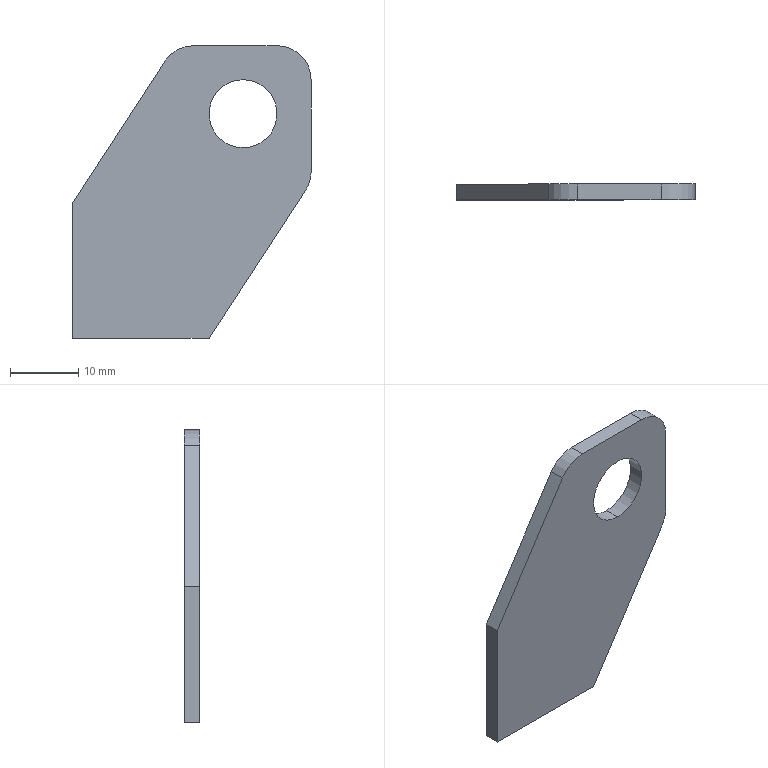Part | SolidWorks | features FlatPattern 1, SMBaseFlange 1, SheetMetal 1 | 1 solid | 13 faces | box 35 x 2.3 x 43 mm | volume 2472 mm3 | plane 8 | cylinder 5 | commonest cylinder face diameters 10 x5
STEP:
#1=CARTESIAN_POINT('',(25.,-2.3,28.));
#2=VERTEX_POINT('',#1);
#3=CARTESIAN_POINT('',(25.,-2.3,38.));
#4=VERTEX_POINT('',#3);
#5=CARTESIAN_POINT('',(25.,-2.3,33.));
#6=DIRECTION('',(0.,1.,0.));
#7=DIRECTION('',(0.,0.,1.));
#8=AXIS2_PLACEMENT_3D('',#5,#6,#7);
#9=CIRCLE('',#8,5.);
#10=EDGE_CURVE('',#2,#4,#9,.T.);
#11=ORIENTED_EDGE('',*,*,#10,.F.);
#12=CARTESIAN_POINT('',(25.,0.,28.));
#13=VERTEX_POINT('',#12);
#14=CARTESIAN_POINT('',(25.,-2.3,28.));
#15=DIRECTION('',(0.,1.,0.));
#16=VECTOR('',#15,1000.);
#17=LINE('',#14,#16);
#18=EDGE_CURVE('',#2,#13,#17,.T.);
#19=ORIENTED_EDGE('',*,*,#18,.T.);
#20=CARTESIAN_POINT('',(25.,0.,38.));
#21=VERTEX_POINT('',#20);
#22=CARTESIAN_POINT('',(25.,0.,33.));
#23=DIRECTION('',(0.,1.,0.));
#24=DIRECTION('',(0.,0.,1.));
#25=AXIS2_PLACEMENT_3D('',#22,#23,#24);
#26=CIRCLE('',#25,5.);
#27=EDGE_CURVE('',#13,#21,#26,.T.);
#28=ORIENTED_EDGE('',*,*,#27,.T.);
#29=CARTESIAN_POINT('',(25.,-2.3,38.));
#30=DIRECTION('',(0.,1.,0.));
#31=VECTOR('',#30,1000.);
#32=LINE('',#29,#31);
#33=EDGE_CURVE('',#4,#21,#32,.T.);
#34=ORIENTED_EDGE('',*,*,#33,.F.);
#35=EDGE_LOOP('',(#11,#19,#28,#34));
#36=FACE_OUTER_BOUND('',#35,.T.);
#37=CARTESIAN_POINT('',(25.,-2.3,33.));
#38=DIRECTION('',(0.,1.,0.));
#39=DIRECTION('',(0.,0.,1.));
#40=AXIS2_PLACEMENT_3D('',#37,#38,#39);
#41=CYLINDRICAL_SURFACE('',#40,5.);
#42=ADVANCED_FACE('',(#36),#41,.F.);
#43=CARTESIAN_POINT('',(0.,0.,0.));
#44=VERTEX_POINT('',#43);
#45=CARTESIAN_POINT('',(0.,0.,20.));
#46=VERTEX_POINT('',#45);
#47=CARTESIAN_POINT('',(0.,0.,0.));
#48=DIRECTION('',(0.,0.,1.));
#49=VECTOR('',#48,1000.);
#50=LINE('',#47,#49);
#51=EDGE_CURVE('',#44,#46,#50,.T.);
#52=ORIENTED_EDGE('',*,*,#51,.F.);
#53=CARTESIAN_POINT('',(0.,-2.3,0.));
#54=VERTEX_POINT('',#53);
#55=CARTESIAN_POINT('',(0.,-2.3,0.));
#56=DIRECTION('',(0.,1.,0.));
#57=VECTOR('',#56,1000.);
#58=LINE('',#55,#57);
#59=EDGE_CURVE('',#54,#44,#58,.T.);
#60=ORIENTED_EDGE('',*,*,#59,.F.);
#61=CARTESIAN_POINT('',(0.,-2.3,20.));
#62=VERTEX_POINT('',#61);
#63=CARTESIAN_POINT('',(0.,-2.3,0.));
#64=DIRECTION('',(0.,0.,1.));
#65=VECTOR('',#64,1000.);
#66=LINE('',#63,#65);
#67=EDGE_CURVE('',#54,#62,#66,.T.);
#68=ORIENTED_EDGE('',*,*,#67,.T.);
#69=CARTESIAN_POINT('',(0.,-2.3,20.));
#70=DIRECTION('',(0.,1.,0.));
#71=VECTOR('',#70,1000.);
#72=LINE('',#69,#71);
#73=EDGE_CURVE('',#62,#46,#72,.T.);
#74=ORIENTED_EDGE('',*,*,#73,.T.);
#75=EDGE_LOOP('',(#52,#60,#68,#74));
#76=FACE_OUTER_BOUND('',#75,.T.);
#77=CARTESIAN_POINT('',(0.,-2.3,0.));
#78=DIRECTION('',(-1.,0.,0.));
#79=DIRECTION('',(0.,0.,1.));
#80=AXIS2_PLACEMENT_3D('',#77,#78,#79);
#81=PLANE('',#80);
#82=ADVANCED_FACE('',(#76),#81,.T.);
#83=CARTESIAN_POINT('',(20.,0.,0.));
#84=VERTEX_POINT('',#83);
#85=CARTESIAN_POINT('',(0.,0.,0.));
#86=DIRECTION('',(-1.,0.,0.));
#87=VECTOR('',#86,1000.);
#88=LINE('',#85,#87);
#89=EDGE_CURVE('',#84,#44,#88,.T.);
#90=ORIENTED_EDGE('',*,*,#89,.F.);
#91=CARTESIAN_POINT('',(20.,-2.3,0.));
#92=VERTEX_POINT('',#91);
#93=CARTESIAN_POINT('',(20.,-2.3,0.));
#94=DIRECTION('',(0.,1.,0.));
#95=VECTOR('',#94,1000.);
#96=LINE('',#93,#95);
#97=EDGE_CURVE('',#92,#84,#96,.T.);
#98=ORIENTED_EDGE('',*,*,#97,.F.);
#99=CARTESIAN_POINT('',(0.,-2.3,0.));
#100=DIRECTION('',(-1.,0.,0.));
#101=VECTOR('',#100,1000.);
#102=LINE('',#99,#101);
#103=EDGE_CURVE('',#92,#54,#102,.T.);
#104=ORIENTED_EDGE('',*,*,#103,.T.);
#105=ORIENTED_EDGE('',*,*,#59,.T.);
#106=EDGE_LOOP('',(#90,#98,#104,#105));
#107=FACE_OUTER_BOUND('',#106,.T.);
#108=CARTESIAN_POINT('',(0.,-2.3,0.));
#109=DIRECTION('',(0.,0.,-1.));
#110=DIRECTION('',(-1.,0.,0.));
#111=AXIS2_PLACEMENT_3D('',#108,#109,#110);
#112=PLANE('',#111);
#113=ADVANCED_FACE('',(#107),#112,.T.);
#114=CARTESIAN_POINT('',(34.188,0.,21.755));
#115=VERTEX_POINT('',#114);
#116=CARTESIAN_POINT('',(20.,0.,0.));
#117=DIRECTION('',(-0.5463,0.,-0.8376));
#118=VECTOR('',#117,1000.);
#119=LINE('',#116,#118);
#120=EDGE_CURVE('',#115,#84,#119,.T.);
#121=ORIENTED_EDGE('',*,*,#120,.F.);
#122=CARTESIAN_POINT('',(34.188,-2.3,21.755));
#123=VERTEX_POINT('',#122);
#124=CARTESIAN_POINT('',(34.188,-2.3,21.755));
#125=DIRECTION('',(0.,1.,0.));
#126=VECTOR('',#125,1000.);
#127=LINE('',#124,#126);
#128=EDGE_CURVE('',#123,#115,#127,.T.);
#129=ORIENTED_EDGE('',*,*,#128,.F.);
#130=CARTESIAN_POINT('',(20.,-2.3,0.));
#131=DIRECTION('',(-0.5463,0.,-0.8376));
#132=VECTOR('',#131,1000.);
#133=LINE('',#130,#132);
#134=EDGE_CURVE('',#123,#92,#133,.T.);
#135=ORIENTED_EDGE('',*,*,#134,.T.);
#136=ORIENTED_EDGE('',*,*,#97,.T.);
#137=EDGE_LOOP('',(#121,#129,#135,#136));
#138=FACE_OUTER_BOUND('',#137,.T.);
#139=CARTESIAN_POINT('',(20.,-2.3,0.));
#140=DIRECTION('',(0.8376,0.,-0.5463));
#141=DIRECTION('',(-0.5463,0.,-0.8376));
#142=AXIS2_PLACEMENT_3D('',#139,#140,#141);
#143=PLANE('',#142);
#144=ADVANCED_FACE('',(#138),#143,.T.);
#145=CARTESIAN_POINT('',(35.,0.,24.486));
#146=VERTEX_POINT('',#145);
#147=CARTESIAN_POINT('',(30.,0.,24.486));
#148=DIRECTION('',(0.,1.,0.));
#149=DIRECTION('',(0.,0.,-1.));
#150=AXIS2_PLACEMENT_3D('',#147,#148,#149);
#151=CIRCLE('',#150,5.);
#152=EDGE_CURVE('',#146,#115,#151,.T.);
#153=ORIENTED_EDGE('',*,*,#152,.F.);
#154=CARTESIAN_POINT('',(35.,-2.3,24.486));
#155=VERTEX_POINT('',#154);
#156=CARTESIAN_POINT('',(35.,-2.3,24.486));
#157=DIRECTION('',(0.,1.,0.));
#158=VECTOR('',#157,1000.);
#159=LINE('',#156,#158);
#160=EDGE_CURVE('',#155,#146,#159,.T.);
#161=ORIENTED_EDGE('',*,*,#160,.F.);
#162=CARTESIAN_POINT('',(30.,-2.3,24.486));
#163=DIRECTION('',(0.,1.,0.));
#164=DIRECTION('',(0.,0.,-1.));
#165=AXIS2_PLACEMENT_3D('',#162,#163,#164);
#166=CIRCLE('',#165,5.);
#167=EDGE_CURVE('',#155,#123,#166,.T.);
#168=ORIENTED_EDGE('',*,*,#167,.T.);
#169=ORIENTED_EDGE('',*,*,#128,.T.);
#170=EDGE_LOOP('',(#153,#161,#168,#169));
#171=FACE_OUTER_BOUND('',#170,.T.);
#172=CARTESIAN_POINT('',(30.,-2.3,24.486));
#173=DIRECTION('',(0.,1.,0.));
#174=DIRECTION('',(0.,0.,1.));
#175=AXIS2_PLACEMENT_3D('',#172,#173,#174);
#176=CYLINDRICAL_SURFACE('',#175,5.);
#177=ADVANCED_FACE('',(#171),#176,.T.);
#178=CARTESIAN_POINT('',(35.,0.,38.));
#179=VERTEX_POINT('',#178);
#180=CARTESIAN_POINT('',(35.,0.,24.486));
#181=DIRECTION('',(0.,0.,-1.));
#182=VECTOR('',#181,1000.);
#183=LINE('',#180,#182);
#184=EDGE_CURVE('',#179,#146,#183,.T.);
#185=ORIENTED_EDGE('',*,*,#184,.F.);
#186=CARTESIAN_POINT('',(35.,-2.3,38.));
#187=VERTEX_POINT('',#186);
#188=CARTESIAN_POINT('',(35.,-2.3,38.));
#189=DIRECTION('',(0.,1.,0.));
#190=VECTOR('',#189,1000.);
#191=LINE('',#188,#190);
#192=EDGE_CURVE('',#187,#179,#191,.T.);
#193=ORIENTED_EDGE('',*,*,#192,.F.);
#194=CARTESIAN_POINT('',(35.,-2.3,24.486));
#195=DIRECTION('',(0.,0.,-1.));
#196=VECTOR('',#195,1000.);
#197=LINE('',#194,#196);
#198=EDGE_CURVE('',#187,#155,#197,.T.);
#199=ORIENTED_EDGE('',*,*,#198,.T.);
#200=ORIENTED_EDGE('',*,*,#160,.T.);
#201=EDGE_LOOP('',(#185,#193,#199,#200));
#202=FACE_OUTER_BOUND('',#201,.T.);
#203=CARTESIAN_POINT('',(35.,-2.3,24.486));
#204=DIRECTION('',(1.,0.,0.));
#205=DIRECTION('',(0.,0.,-1.));
#206=AXIS2_PLACEMENT_3D('',#203,#204,#205);
#207=PLANE('',#206);
#208=ADVANCED_FACE('',(#202),#207,.T.);
#209=CARTESIAN_POINT('',(30.,0.,43.));
#210=VERTEX_POINT('',#209);
#211=CARTESIAN_POINT('',(30.,0.,38.));
#212=DIRECTION('',(0.,1.,0.));
#213=DIRECTION('',(0.,0.,1.));
#214=AXIS2_PLACEMENT_3D('',#211,#212,#213);
#215=CIRCLE('',#214,5.);
#216=EDGE_CURVE('',#210,#179,#215,.T.);
#217=ORIENTED_EDGE('',*,*,#216,.F.);
#218=CARTESIAN_POINT('',(30.,-2.3,43.));
#219=VERTEX_POINT('',#218);
#220=CARTESIAN_POINT('',(30.,-2.3,43.));
#221=DIRECTION('',(0.,1.,0.));
#222=VECTOR('',#221,1000.);
#223=LINE('',#220,#222);
#224=EDGE_CURVE('',#219,#210,#223,.T.);
#225=ORIENTED_EDGE('',*,*,#224,.F.);
#226=CARTESIAN_POINT('',(30.,-2.3,38.));
#227=DIRECTION('',(0.,1.,0.));
#228=DIRECTION('',(0.,0.,1.));
#229=AXIS2_PLACEMENT_3D('',#226,#227,#228);
#230=CIRCLE('',#229,5.);
#231=EDGE_CURVE('',#219,#187,#230,.T.);
#232=ORIENTED_EDGE('',*,*,#231,.T.);
#233=ORIENTED_EDGE('',*,*,#192,.T.);
#234=EDGE_LOOP('',(#217,#225,#232,#233));
#235=FACE_OUTER_BOUND('',#234,.T.);
#236=CARTESIAN_POINT('',(30.,-2.3,38.));
#237=DIRECTION('',(0.,1.,0.));
#238=DIRECTION('',(0.,0.,1.));
#239=AXIS2_PLACEMENT_3D('',#236,#237,#238);
#240=CYLINDRICAL_SURFACE('',#239,5.);
#241=ADVANCED_FACE('',(#235),#240,.T.);
#242=CARTESIAN_POINT('',(17.708,0.,43.));
#243=VERTEX_POINT('',#242);
#244=CARTESIAN_POINT('',(17.708,0.,43.));
#245=DIRECTION('',(1.,0.,0.));
#246=VECTOR('',#245,1000.);
#247=LINE('',#244,#246);
#248=EDGE_CURVE('',#243,#210,#247,.T.);
#249=ORIENTED_EDGE('',*,*,#248,.F.);
#250=CARTESIAN_POINT('',(17.708,-2.3,43.));
#251=VERTEX_POINT('',#250);
#252=CARTESIAN_POINT('',(17.708,-2.3,43.));
#253=DIRECTION('',(0.,1.,0.));
#254=VECTOR('',#253,1000.);
#255=LINE('',#252,#254);
#256=EDGE_CURVE('',#251,#243,#255,.T.);
#257=ORIENTED_EDGE('',*,*,#256,.F.);
#258=CARTESIAN_POINT('',(17.708,-2.3,43.));
#259=DIRECTION('',(1.,0.,0.));
#260=VECTOR('',#259,1000.);
#261=LINE('',#258,#260);
#262=EDGE_CURVE('',#251,#219,#261,.T.);
#263=ORIENTED_EDGE('',*,*,#262,.T.);
#264=ORIENTED_EDGE('',*,*,#224,.T.);
#265=EDGE_LOOP('',(#249,#257,#263,#264));
#266=FACE_OUTER_BOUND('',#265,.T.);
#267=CARTESIAN_POINT('',(17.708,-2.3,43.));
#268=DIRECTION('',(0.,0.,1.));
#269=DIRECTION('',(1.,0.,0.));
#270=AXIS2_PLACEMENT_3D('',#267,#268,#269);
#271=PLANE('',#270);
#272=ADVANCED_FACE('',(#266),#271,.T.);
#273=CARTESIAN_POINT('',(13.52,0.,40.731));
#274=VERTEX_POINT('',#273);
#275=CARTESIAN_POINT('',(17.708,0.,38.));
#276=DIRECTION('',(0.,1.,0.));
#277=DIRECTION('',(0.,0.,-1.));
#278=AXIS2_PLACEMENT_3D('',#275,#276,#277);
#279=CIRCLE('',#278,5.);
#280=EDGE_CURVE('',#274,#243,#279,.T.);
#281=ORIENTED_EDGE('',*,*,#280,.F.);
#282=CARTESIAN_POINT('',(13.52,-2.3,40.731));
#283=VERTEX_POINT('',#282);
#284=CARTESIAN_POINT('',(13.52,-2.3,40.731));
#285=DIRECTION('',(0.,1.,0.));
#286=VECTOR('',#285,1000.);
#287=LINE('',#284,#286);
#288=EDGE_CURVE('',#283,#274,#287,.T.);
#289=ORIENTED_EDGE('',*,*,#288,.F.);
#290=CARTESIAN_POINT('',(17.708,-2.3,38.));
#291=DIRECTION('',(0.,1.,0.));
#292=DIRECTION('',(0.,0.,-1.));
#293=AXIS2_PLACEMENT_3D('',#290,#291,#292);
#294=CIRCLE('',#293,5.);
#295=EDGE_CURVE('',#283,#251,#294,.T.);
#296=ORIENTED_EDGE('',*,*,#295,.T.);
#297=ORIENTED_EDGE('',*,*,#256,.T.);
#298=EDGE_LOOP('',(#281,#289,#296,#297));
#299=FACE_OUTER_BOUND('',#298,.T.);
#300=CARTESIAN_POINT('',(17.708,-2.3,38.));
#301=DIRECTION('',(0.,1.,0.));
#302=DIRECTION('',(0.,0.,1.));
#303=AXIS2_PLACEMENT_3D('',#300,#301,#302);
#304=CYLINDRICAL_SURFACE('',#303,5.);
#305=ADVANCED_FACE('',(#299),#304,.T.);
#306=CARTESIAN_POINT('',(0.,0.,20.));
#307=DIRECTION('',(0.5463,0.,0.8376));
#308=VECTOR('',#307,1000.);
#309=LINE('',#306,#308);
#310=EDGE_CURVE('',#46,#274,#309,.T.);
#311=ORIENTED_EDGE('',*,*,#310,.F.);
#312=ORIENTED_EDGE('',*,*,#73,.F.);
#313=CARTESIAN_POINT('',(0.,-2.3,20.));
#314=DIRECTION('',(0.5463,0.,0.8376));
#315=VECTOR('',#314,1000.);
#316=LINE('',#313,#315);
#317=EDGE_CURVE('',#62,#283,#316,.T.);
#318=ORIENTED_EDGE('',*,*,#317,.T.);
#319=ORIENTED_EDGE('',*,*,#288,.T.);
#320=EDGE_LOOP('',(#311,#312,#318,#319));
#321=FACE_OUTER_BOUND('',#320,.T.);
#322=CARTESIAN_POINT('',(0.,-2.3,20.));
#323=DIRECTION('',(-0.8376,0.,0.5463));
#324=DIRECTION('',(0.5463,0.,0.8376));
#325=AXIS2_PLACEMENT_3D('',#322,#323,#324);
#326=PLANE('',#325);
#327=ADVANCED_FACE('',(#321),#326,.T.);
#328=CARTESIAN_POINT('',(25.,-2.3,33.));
#329=DIRECTION('',(0.,1.,0.));
#330=DIRECTION('',(0.,0.,1.));
#331=AXIS2_PLACEMENT_3D('',#328,#329,#330);
#332=CIRCLE('',#331,5.);
#333=EDGE_CURVE('',#4,#2,#332,.T.);
#334=ORIENTED_EDGE('',*,*,#333,.T.);
#335=ORIENTED_EDGE('',*,*,#10,.T.);
#336=EDGE_LOOP('',(#334,#335));
#337=FACE_BOUND('',#336,.T.);
#338=ORIENTED_EDGE('',*,*,#67,.F.);
#339=ORIENTED_EDGE('',*,*,#103,.F.);
#340=ORIENTED_EDGE('',*,*,#134,.F.);
#341=ORIENTED_EDGE('',*,*,#167,.F.);
#342=ORIENTED_EDGE('',*,*,#198,.F.);
#343=ORIENTED_EDGE('',*,*,#231,.F.);
#344=ORIENTED_EDGE('',*,*,#262,.F.);
#345=ORIENTED_EDGE('',*,*,#295,.F.);
#346=ORIENTED_EDGE('',*,*,#317,.F.);
#347=EDGE_LOOP('',(#338,#339,#340,#341,#342,#343,#344,#345,#346));
#348=FACE_OUTER_BOUND('',#347,.T.);
#349=CARTESIAN_POINT('',(17.708,-2.3,38.));
#350=DIRECTION('',(0.,-1.,0.));
#351=DIRECTION('',(0.,0.,-1.));
#352=AXIS2_PLACEMENT_3D('',#349,#350,#351);
#353=PLANE('',#352);
#354=ADVANCED_FACE('',(#337,#348),#353,.T.);
#355=CARTESIAN_POINT('',(25.,0.,33.));
#356=DIRECTION('',(0.,1.,0.));
#357=DIRECTION('',(0.,0.,1.));
#358=AXIS2_PLACEMENT_3D('',#355,#356,#357);
#359=CIRCLE('',#358,5.);
#360=EDGE_CURVE('',#21,#13,#359,.T.);
#361=ORIENTED_EDGE('',*,*,#360,.F.);
#362=ORIENTED_EDGE('',*,*,#27,.F.);
#363=EDGE_LOOP('',(#361,#362));
#364=FACE_BOUND('',#363,.T.);
#365=ORIENTED_EDGE('',*,*,#51,.T.);
#366=ORIENTED_EDGE('',*,*,#310,.T.);
#367=ORIENTED_EDGE('',*,*,#280,.T.);
#368=ORIENTED_EDGE('',*,*,#248,.T.);
#369=ORIENTED_EDGE('',*,*,#216,.T.);
#370=ORIENTED_EDGE('',*,*,#184,.T.);
#371=ORIENTED_EDGE('',*,*,#152,.T.);
#372=ORIENTED_EDGE('',*,*,#120,.T.);
#373=ORIENTED_EDGE('',*,*,#89,.T.);
#374=EDGE_LOOP('',(#365,#366,#367,#368,#369,#370,#371,#372,#373));
#375=FACE_OUTER_BOUND('',#374,.T.);
#376=CARTESIAN_POINT('',(17.708,0.,38.));
#377=DIRECTION('',(0.,-1.,0.));
#378=DIRECTION('',(0.,0.,-1.));
#379=AXIS2_PLACEMENT_3D('',#376,#377,#378);
#380=PLANE('',#379);
#381=ADVANCED_FACE('',(#364,#375),#380,.F.);
#382=ORIENTED_EDGE('',*,*,#18,.F.);
#383=ORIENTED_EDGE('',*,*,#333,.F.);
#384=ORIENTED_EDGE('',*,*,#33,.T.);
#385=ORIENTED_EDGE('',*,*,#360,.T.);
#386=EDGE_LOOP('',(#382,#383,#384,#385));
#387=FACE_OUTER_BOUND('',#386,.T.);
#388=CARTESIAN_POINT('',(25.,-2.3,33.));
#389=DIRECTION('',(0.,1.,0.));
#390=DIRECTION('',(0.,0.,1.));
#391=AXIS2_PLACEMENT_3D('',#388,#389,#390);
#392=CYLINDRICAL_SURFACE('',#391,5.);
#393=ADVANCED_FACE('',(#387),#392,.F.);
#394=CLOSED_SHELL('',(#42,#82,#113,#144,#177,#208,#241,#272,#305,#327,#354,#381,#393));
#395=MANIFOLD_SOLID_BREP('',#394);
#396=CARTESIAN_POINT('',(0.,0.,0.));
#397=DIRECTION('',(0.,0.,1.));
#398=DIRECTION('',(1.,0.,0.));
#399=AXIS2_PLACEMENT_3D('',#396,#397,#398);
#400=(LENGTH_UNIT()NAMED_UNIT(*)SI_UNIT(.MILLI.,.METRE.));
#401=UNCERTAINTY_MEASURE_WITH_UNIT(LENGTH_MEASURE(0.00001),#400,'','');
#402=(NAMED_UNIT(*)PLANE_ANGLE_UNIT()SI_UNIT($,.RADIAN.));
#403=(NAMED_UNIT(*)SI_UNIT($,.STERADIAN.)SOLID_ANGLE_UNIT());
#404=(GEOMETRIC_REPRESENTATION_CONTEXT(3)GLOBAL_UNCERTAINTY_ASSIGNED_CONTEXT((#401))GLOBAL_UNIT_ASSIGNED_CONTEXT((#400,#402,#403))REPRESENTATION_CONTEXT('',''));
#405=ADVANCED_BREP_SHAPE_REPRESENTATION('',(#395,#399),#404);